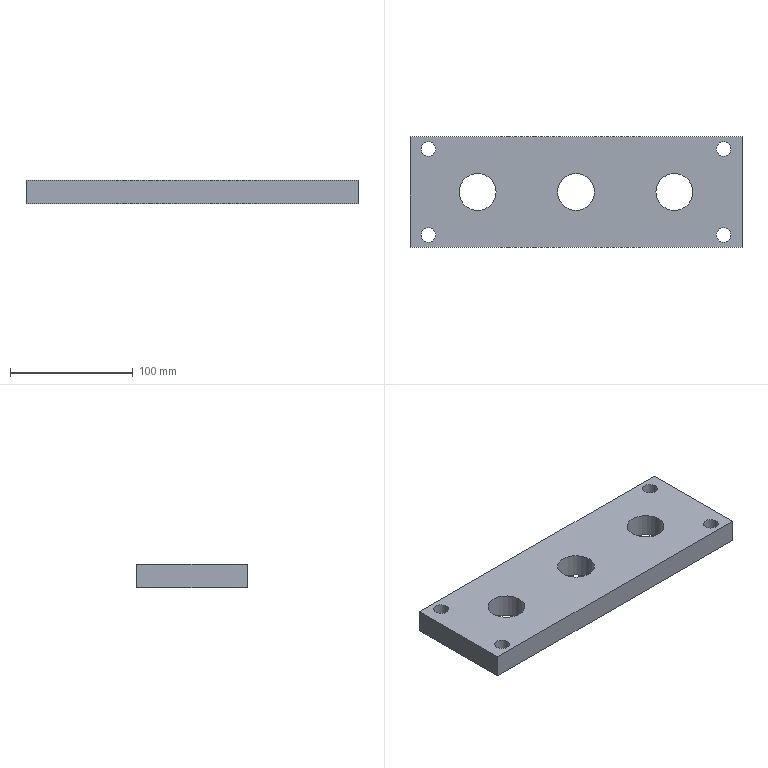Part | NX | features solid 2 | 1 solid | 13 faces | box 270 x 90 x 19 mm | volume 412814 mm3 | cylinder 7 | plane 6 | commonest cylinder face diameters 12 x4 30 x3
STEP:
#1=CARTESIAN_POINT('',(114.,-405.,-144.));
#2=VERTEX_POINT('',#1);
#3=CARTESIAN_POINT('',(120.,-405.,-144.));
#4=DIRECTION('',(0.,0.,1.));
#5=DIRECTION('',(-1.,0.,0.));
#6=AXIS2_PLACEMENT_3D('',#3,#4,#5);
#7=CIRCLE('',#6,6.);
#8=EDGE_CURVE('',#2,#2,#7,.T.);
#9=ORIENTED_EDGE('',*,*,#8,.T.);
#10=EDGE_LOOP('',(#9));
#11=FACE_BOUND('',#10,.T.);
#12=CARTESIAN_POINT('',(114.,-475.,-144.));
#13=VERTEX_POINT('',#12);
#14=CARTESIAN_POINT('',(120.,-475.,-144.));
#15=DIRECTION('',(0.,0.,-1.));
#16=DIRECTION('',(-1.,0.,0.));
#17=AXIS2_PLACEMENT_3D('',#14,#15,#16);
#18=CIRCLE('',#17,6.);
#19=EDGE_CURVE('',#13,#13,#18,.T.);
#20=ORIENTED_EDGE('',*,*,#19,.F.);
#21=EDGE_LOOP('',(#20));
#22=FACE_BOUND('',#21,.T.);
#23=CARTESIAN_POINT('',(-114.,-405.,-144.));
#24=VERTEX_POINT('',#23);
#25=CARTESIAN_POINT('',(-120.,-405.,-144.));
#26=DIRECTION('',(0.,0.,-1.));
#27=DIRECTION('',(1.,0.,0.));
#28=AXIS2_PLACEMENT_3D('',#25,#26,#27);
#29=CIRCLE('',#28,6.);
#30=EDGE_CURVE('',#24,#24,#29,.T.);
#31=ORIENTED_EDGE('',*,*,#30,.F.);
#32=EDGE_LOOP('',(#31));
#33=FACE_BOUND('',#32,.T.);
#34=CARTESIAN_POINT('',(95.,-440.,-144.));
#35=VERTEX_POINT('',#34);
#36=CARTESIAN_POINT('',(80.,-440.,-144.));
#37=DIRECTION('',(0.,0.,-1.));
#38=DIRECTION('',(1.,0.,0.));
#39=AXIS2_PLACEMENT_3D('',#36,#37,#38);
#40=CIRCLE('',#39,15.);
#41=EDGE_CURVE('',#35,#35,#40,.T.);
#42=ORIENTED_EDGE('',*,*,#41,.F.);
#43=EDGE_LOOP('',(#42));
#44=FACE_BOUND('',#43,.T.);
#45=CARTESIAN_POINT('',(-15.,-440.,-144.));
#46=VERTEX_POINT('',#45);
#47=CARTESIAN_POINT('',(0.,-440.,-144.));
#48=DIRECTION('',(0.,0.,1.));
#49=DIRECTION('',(-1.,0.,0.));
#50=AXIS2_PLACEMENT_3D('',#47,#48,#49);
#51=CIRCLE('',#50,15.);
#52=EDGE_CURVE('',#46,#46,#51,.T.);
#53=ORIENTED_EDGE('',*,*,#52,.T.);
#54=EDGE_LOOP('',(#53));
#55=FACE_BOUND('',#54,.T.);
#56=CARTESIAN_POINT('',(-135.,-485.,-144.));
#57=VERTEX_POINT('',#56);
#58=CARTESIAN_POINT('',(-135.,-395.,-144.));
#59=VERTEX_POINT('',#58);
#60=CARTESIAN_POINT('',(-135.,-485.,-144.));
#61=DIRECTION('',(0.,1.,0.));
#62=VECTOR('',#61,1000.);
#63=LINE('',#60,#62);
#64=EDGE_CURVE('',#57,#59,#63,.T.);
#65=ORIENTED_EDGE('',*,*,#64,.T.);
#66=CARTESIAN_POINT('',(135.,-395.,-144.));
#67=VERTEX_POINT('',#66);
#68=CARTESIAN_POINT('',(-135.,-395.,-144.));
#69=DIRECTION('',(1.,0.,0.));
#70=VECTOR('',#69,1000.);
#71=LINE('',#68,#70);
#72=EDGE_CURVE('',#59,#67,#71,.T.);
#73=ORIENTED_EDGE('',*,*,#72,.T.);
#74=CARTESIAN_POINT('',(135.,-485.,-144.));
#75=VERTEX_POINT('',#74);
#76=CARTESIAN_POINT('',(135.,-395.,-144.));
#77=DIRECTION('',(0.,-1.,0.));
#78=VECTOR('',#77,1000.);
#79=LINE('',#76,#78);
#80=EDGE_CURVE('',#67,#75,#79,.T.);
#81=ORIENTED_EDGE('',*,*,#80,.T.);
#82=CARTESIAN_POINT('',(135.,-485.,-144.));
#83=DIRECTION('',(-1.,0.,0.));
#84=VECTOR('',#83,1000.);
#85=LINE('',#82,#84);
#86=EDGE_CURVE('',#75,#57,#85,.T.);
#87=ORIENTED_EDGE('',*,*,#86,.T.);
#88=EDGE_LOOP('',(#65,#73,#81,#87));
#89=FACE_BOUND('',#88,.T.);
#90=CARTESIAN_POINT('',(-95.,-440.,-144.));
#91=VERTEX_POINT('',#90);
#92=CARTESIAN_POINT('',(-80.,-440.,-144.));
#93=DIRECTION('',(0.,0.,1.));
#94=DIRECTION('',(-1.,0.,0.));
#95=AXIS2_PLACEMENT_3D('',#92,#93,#94);
#96=CIRCLE('',#95,15.);
#97=EDGE_CURVE('',#91,#91,#96,.T.);
#98=ORIENTED_EDGE('',*,*,#97,.T.);
#99=EDGE_LOOP('',(#98));
#100=FACE_BOUND('',#99,.T.);
#101=CARTESIAN_POINT('',(-114.,-475.,-144.));
#102=VERTEX_POINT('',#101);
#103=CARTESIAN_POINT('',(-120.,-475.,-144.));
#104=DIRECTION('',(0.,0.,1.));
#105=DIRECTION('',(1.,0.,0.));
#106=AXIS2_PLACEMENT_3D('',#103,#104,#105);
#107=CIRCLE('',#106,6.);
#108=EDGE_CURVE('',#102,#102,#107,.T.);
#109=ORIENTED_EDGE('',*,*,#108,.T.);
#110=EDGE_LOOP('',(#109));
#111=FACE_BOUND('',#110,.T.);
#112=CARTESIAN_POINT('',(-135.,-395.,-144.));
#113=DIRECTION('',(0.,0.,1.));
#114=DIRECTION('',(-1.,0.,0.));
#115=AXIS2_PLACEMENT_3D('',#112,#113,#114);
#116=PLANE('',#115);
#117=ADVANCED_FACE('',(#11,#22,#33,#44,#55,#89,#100,#111),#116,.F.);
#118=CARTESIAN_POINT('',(114.,-405.,-125.));
#119=VERTEX_POINT('',#118);
#120=CARTESIAN_POINT('',(120.,-405.,-125.));
#121=DIRECTION('',(0.,0.,1.));
#122=DIRECTION('',(-1.,0.,0.));
#123=AXIS2_PLACEMENT_3D('',#120,#121,#122);
#124=CIRCLE('',#123,6.);
#125=EDGE_CURVE('',#119,#119,#124,.T.);
#126=ORIENTED_EDGE('',*,*,#125,.F.);
#127=EDGE_LOOP('',(#126));
#128=FACE_BOUND('',#127,.T.);
#129=CARTESIAN_POINT('',(114.,-475.,-125.));
#130=VERTEX_POINT('',#129);
#131=CARTESIAN_POINT('',(120.,-475.,-125.));
#132=DIRECTION('',(0.,0.,-1.));
#133=DIRECTION('',(-1.,0.,0.));
#134=AXIS2_PLACEMENT_3D('',#131,#132,#133);
#135=CIRCLE('',#134,6.);
#136=EDGE_CURVE('',#130,#130,#135,.T.);
#137=ORIENTED_EDGE('',*,*,#136,.T.);
#138=EDGE_LOOP('',(#137));
#139=FACE_BOUND('',#138,.T.);
#140=CARTESIAN_POINT('',(-114.,-405.,-125.));
#141=VERTEX_POINT('',#140);
#142=CARTESIAN_POINT('',(-120.,-405.,-125.));
#143=DIRECTION('',(0.,0.,-1.));
#144=DIRECTION('',(1.,0.,0.));
#145=AXIS2_PLACEMENT_3D('',#142,#143,#144);
#146=CIRCLE('',#145,6.);
#147=EDGE_CURVE('',#141,#141,#146,.T.);
#148=ORIENTED_EDGE('',*,*,#147,.T.);
#149=EDGE_LOOP('',(#148));
#150=FACE_BOUND('',#149,.T.);
#151=CARTESIAN_POINT('',(95.,-440.,-125.));
#152=VERTEX_POINT('',#151);
#153=CARTESIAN_POINT('',(80.,-440.,-125.));
#154=DIRECTION('',(0.,0.,-1.));
#155=DIRECTION('',(1.,0.,0.));
#156=AXIS2_PLACEMENT_3D('',#153,#154,#155);
#157=CIRCLE('',#156,15.);
#158=EDGE_CURVE('',#152,#152,#157,.T.);
#159=ORIENTED_EDGE('',*,*,#158,.T.);
#160=EDGE_LOOP('',(#159));
#161=FACE_BOUND('',#160,.T.);
#162=CARTESIAN_POINT('',(-15.,-440.,-125.));
#163=VERTEX_POINT('',#162);
#164=CARTESIAN_POINT('',(0.,-440.,-125.));
#165=DIRECTION('',(0.,0.,1.));
#166=DIRECTION('',(-1.,0.,0.));
#167=AXIS2_PLACEMENT_3D('',#164,#165,#166);
#168=CIRCLE('',#167,15.);
#169=EDGE_CURVE('',#163,#163,#168,.T.);
#170=ORIENTED_EDGE('',*,*,#169,.F.);
#171=EDGE_LOOP('',(#170));
#172=FACE_BOUND('',#171,.T.);
#173=CARTESIAN_POINT('',(-135.,-485.,-125.));
#174=VERTEX_POINT('',#173);
#175=CARTESIAN_POINT('',(-135.,-395.,-125.));
#176=VERTEX_POINT('',#175);
#177=CARTESIAN_POINT('',(-135.,-485.,-125.));
#178=DIRECTION('',(0.,1.,0.));
#179=VECTOR('',#178,1000.);
#180=LINE('',#177,#179);
#181=EDGE_CURVE('',#174,#176,#180,.T.);
#182=ORIENTED_EDGE('',*,*,#181,.F.);
#183=CARTESIAN_POINT('',(135.,-485.,-125.));
#184=VERTEX_POINT('',#183);
#185=CARTESIAN_POINT('',(135.,-485.,-125.));
#186=DIRECTION('',(-1.,0.,0.));
#187=VECTOR('',#186,1000.);
#188=LINE('',#185,#187);
#189=EDGE_CURVE('',#184,#174,#188,.T.);
#190=ORIENTED_EDGE('',*,*,#189,.F.);
#191=CARTESIAN_POINT('',(135.,-395.,-125.));
#192=VERTEX_POINT('',#191);
#193=CARTESIAN_POINT('',(135.,-395.,-125.));
#194=DIRECTION('',(0.,-1.,0.));
#195=VECTOR('',#194,1000.);
#196=LINE('',#193,#195);
#197=EDGE_CURVE('',#192,#184,#196,.T.);
#198=ORIENTED_EDGE('',*,*,#197,.F.);
#199=CARTESIAN_POINT('',(-135.,-395.,-125.));
#200=DIRECTION('',(1.,0.,0.));
#201=VECTOR('',#200,1000.);
#202=LINE('',#199,#201);
#203=EDGE_CURVE('',#176,#192,#202,.T.);
#204=ORIENTED_EDGE('',*,*,#203,.F.);
#205=EDGE_LOOP('',(#182,#190,#198,#204));
#206=FACE_BOUND('',#205,.T.);
#207=CARTESIAN_POINT('',(-95.,-440.,-125.));
#208=VERTEX_POINT('',#207);
#209=CARTESIAN_POINT('',(-80.,-440.,-125.));
#210=DIRECTION('',(0.,0.,1.));
#211=DIRECTION('',(-1.,0.,0.));
#212=AXIS2_PLACEMENT_3D('',#209,#210,#211);
#213=CIRCLE('',#212,15.);
#214=EDGE_CURVE('',#208,#208,#213,.T.);
#215=ORIENTED_EDGE('',*,*,#214,.F.);
#216=EDGE_LOOP('',(#215));
#217=FACE_BOUND('',#216,.T.);
#218=CARTESIAN_POINT('',(-114.,-475.,-125.));
#219=VERTEX_POINT('',#218);
#220=CARTESIAN_POINT('',(-120.,-475.,-125.));
#221=DIRECTION('',(0.,0.,1.));
#222=DIRECTION('',(1.,0.,0.));
#223=AXIS2_PLACEMENT_3D('',#220,#221,#222);
#224=CIRCLE('',#223,6.);
#225=EDGE_CURVE('',#219,#219,#224,.T.);
#226=ORIENTED_EDGE('',*,*,#225,.F.);
#227=EDGE_LOOP('',(#226));
#228=FACE_BOUND('',#227,.T.);
#229=CARTESIAN_POINT('',(-135.,-395.,-125.));
#230=DIRECTION('',(0.,0.,1.));
#231=DIRECTION('',(-1.,0.,0.));
#232=AXIS2_PLACEMENT_3D('',#229,#230,#231);
#233=PLANE('',#232);
#234=ADVANCED_FACE('',(#128,#139,#150,#161,#172,#206,#217,#228),#233,.T.);
#235=ORIENTED_EDGE('',*,*,#181,.T.);
#236=CARTESIAN_POINT('',(-135.,-395.,-144.));
#237=DIRECTION('',(0.,0.,1.));
#238=VECTOR('',#237,1000.);
#239=LINE('',#236,#238);
#240=EDGE_CURVE('',#59,#176,#239,.T.);
#241=ORIENTED_EDGE('',*,*,#240,.F.);
#242=ORIENTED_EDGE('',*,*,#64,.F.);
#243=CARTESIAN_POINT('',(-135.,-485.,-144.));
#244=DIRECTION('',(0.,0.,1.));
#245=VECTOR('',#244,1000.);
#246=LINE('',#243,#245);
#247=EDGE_CURVE('',#57,#174,#246,.T.);
#248=ORIENTED_EDGE('',*,*,#247,.T.);
#249=EDGE_LOOP('',(#235,#241,#242,#248));
#250=FACE_BOUND('',#249,.T.);
#251=CARTESIAN_POINT('',(-135.,-485.,-144.));
#252=DIRECTION('',(-1.,0.,0.));
#253=DIRECTION('',(0.,0.,-1.));
#254=AXIS2_PLACEMENT_3D('',#251,#252,#253);
#255=PLANE('',#254);
#256=ADVANCED_FACE('',(#250),#255,.T.);
#257=ORIENTED_EDGE('',*,*,#203,.T.);
#258=CARTESIAN_POINT('',(135.,-395.,-144.));
#259=DIRECTION('',(0.,0.,1.));
#260=VECTOR('',#259,1000.);
#261=LINE('',#258,#260);
#262=EDGE_CURVE('',#67,#192,#261,.T.);
#263=ORIENTED_EDGE('',*,*,#262,.F.);
#264=ORIENTED_EDGE('',*,*,#72,.F.);
#265=ORIENTED_EDGE('',*,*,#240,.T.);
#266=EDGE_LOOP('',(#257,#263,#264,#265));
#267=FACE_BOUND('',#266,.T.);
#268=CARTESIAN_POINT('',(-135.,-395.,-144.));
#269=DIRECTION('',(0.,1.,0.));
#270=DIRECTION('',(0.,0.,-1.));
#271=AXIS2_PLACEMENT_3D('',#268,#269,#270);
#272=PLANE('',#271);
#273=ADVANCED_FACE('',(#267),#272,.T.);
#274=ORIENTED_EDGE('',*,*,#197,.T.);
#275=CARTESIAN_POINT('',(135.,-485.,-144.));
#276=DIRECTION('',(0.,0.,1.));
#277=VECTOR('',#276,1000.);
#278=LINE('',#275,#277);
#279=EDGE_CURVE('',#75,#184,#278,.T.);
#280=ORIENTED_EDGE('',*,*,#279,.F.);
#281=ORIENTED_EDGE('',*,*,#80,.F.);
#282=ORIENTED_EDGE('',*,*,#262,.T.);
#283=EDGE_LOOP('',(#274,#280,#281,#282));
#284=FACE_BOUND('',#283,.T.);
#285=CARTESIAN_POINT('',(135.,-395.,-144.));
#286=DIRECTION('',(1.,0.,0.));
#287=DIRECTION('',(0.,0.,1.));
#288=AXIS2_PLACEMENT_3D('',#285,#286,#287);
#289=PLANE('',#288);
#290=ADVANCED_FACE('',(#284),#289,.T.);
#291=ORIENTED_EDGE('',*,*,#189,.T.);
#292=ORIENTED_EDGE('',*,*,#247,.F.);
#293=ORIENTED_EDGE('',*,*,#86,.F.);
#294=ORIENTED_EDGE('',*,*,#279,.T.);
#295=EDGE_LOOP('',(#291,#292,#293,#294));
#296=FACE_BOUND('',#295,.T.);
#297=CARTESIAN_POINT('',(135.,-485.,-144.));
#298=DIRECTION('',(0.,-1.,0.));
#299=DIRECTION('',(0.,0.,1.));
#300=AXIS2_PLACEMENT_3D('',#297,#298,#299);
#301=PLANE('',#300);
#302=ADVANCED_FACE('',(#296),#301,.T.);
#303=ORIENTED_EDGE('',*,*,#52,.F.);
#304=EDGE_LOOP('',(#303));
#305=FACE_BOUND('',#304,.T.);
#306=ORIENTED_EDGE('',*,*,#169,.T.);
#307=EDGE_LOOP('',(#306));
#308=FACE_BOUND('',#307,.T.);
#309=CARTESIAN_POINT('',(0.,-440.,-144.));
#310=DIRECTION('',(0.,0.,1.));
#311=DIRECTION('',(-1.,0.,0.));
#312=AXIS2_PLACEMENT_3D('',#309,#310,#311);
#313=CYLINDRICAL_SURFACE('',#312,15.);
#314=ADVANCED_FACE('',(#305,#308),#313,.F.);
#315=ORIENTED_EDGE('',*,*,#41,.T.);
#316=EDGE_LOOP('',(#315));
#317=FACE_BOUND('',#316,.T.);
#318=ORIENTED_EDGE('',*,*,#158,.F.);
#319=EDGE_LOOP('',(#318));
#320=FACE_BOUND('',#319,.T.);
#321=CARTESIAN_POINT('',(80.,-440.,-144.));
#322=DIRECTION('',(0.,0.,1.));
#323=DIRECTION('',(-1.,0.,0.));
#324=AXIS2_PLACEMENT_3D('',#321,#322,#323);
#325=CYLINDRICAL_SURFACE('',#324,15.);
#326=ADVANCED_FACE('',(#317,#320),#325,.F.);
#327=ORIENTED_EDGE('',*,*,#97,.F.);
#328=EDGE_LOOP('',(#327));
#329=FACE_BOUND('',#328,.T.);
#330=ORIENTED_EDGE('',*,*,#214,.T.);
#331=EDGE_LOOP('',(#330));
#332=FACE_BOUND('',#331,.T.);
#333=CARTESIAN_POINT('',(-80.,-440.,-144.));
#334=DIRECTION('',(0.,0.,1.));
#335=DIRECTION('',(-1.,0.,0.));
#336=AXIS2_PLACEMENT_3D('',#333,#334,#335);
#337=CYLINDRICAL_SURFACE('',#336,15.);
#338=ADVANCED_FACE('',(#329,#332),#337,.F.);
#339=ORIENTED_EDGE('',*,*,#30,.T.);
#340=EDGE_LOOP('',(#339));
#341=FACE_BOUND('',#340,.T.);
#342=ORIENTED_EDGE('',*,*,#147,.F.);
#343=EDGE_LOOP('',(#342));
#344=FACE_BOUND('',#343,.T.);
#345=CARTESIAN_POINT('',(-120.,-405.,-144.));
#346=DIRECTION('',(0.,0.,1.));
#347=DIRECTION('',(-1.,0.,0.));
#348=AXIS2_PLACEMENT_3D('',#345,#346,#347);
#349=CYLINDRICAL_SURFACE('',#348,6.);
#350=ADVANCED_FACE('',(#341,#344),#349,.F.);
#351=ORIENTED_EDGE('',*,*,#19,.T.);
#352=EDGE_LOOP('',(#351));
#353=FACE_BOUND('',#352,.T.);
#354=ORIENTED_EDGE('',*,*,#136,.F.);
#355=EDGE_LOOP('',(#354));
#356=FACE_BOUND('',#355,.T.);
#357=CARTESIAN_POINT('',(120.,-475.,-144.));
#358=DIRECTION('',(0.,0.,1.));
#359=DIRECTION('',(-1.,0.,0.));
#360=AXIS2_PLACEMENT_3D('',#357,#358,#359);
#361=CYLINDRICAL_SURFACE('',#360,6.);
#362=ADVANCED_FACE('',(#353,#356),#361,.F.);
#363=ORIENTED_EDGE('',*,*,#8,.F.);
#364=EDGE_LOOP('',(#363));
#365=FACE_BOUND('',#364,.T.);
#366=ORIENTED_EDGE('',*,*,#125,.T.);
#367=EDGE_LOOP('',(#366));
#368=FACE_BOUND('',#367,.T.);
#369=CARTESIAN_POINT('',(120.,-405.,-144.));
#370=DIRECTION('',(0.,0.,1.));
#371=DIRECTION('',(-1.,0.,0.));
#372=AXIS2_PLACEMENT_3D('',#369,#370,#371);
#373=CYLINDRICAL_SURFACE('',#372,6.);
#374=ADVANCED_FACE('',(#365,#368),#373,.F.);
#375=ORIENTED_EDGE('',*,*,#108,.F.);
#376=EDGE_LOOP('',(#375));
#377=FACE_BOUND('',#376,.T.);
#378=ORIENTED_EDGE('',*,*,#225,.T.);
#379=EDGE_LOOP('',(#378));
#380=FACE_BOUND('',#379,.T.);
#381=CARTESIAN_POINT('',(-120.,-475.,-144.));
#382=DIRECTION('',(0.,0.,1.));
#383=DIRECTION('',(-1.,0.,0.));
#384=AXIS2_PLACEMENT_3D('',#381,#382,#383);
#385=CYLINDRICAL_SURFACE('',#384,6.);
#386=ADVANCED_FACE('',(#377,#380),#385,.F.);
#387=CLOSED_SHELL('',(#117,#234,#256,#273,#290,#302,#314,#326,#338,#350,#362,#374,#386));
#388=MANIFOLD_SOLID_BREP('',#387);
#389=(LENGTH_UNIT()NAMED_UNIT(*)SI_UNIT(.MILLI.,.METRE.));
#390=UNCERTAINTY_MEASURE_WITH_UNIT(LENGTH_MEASURE(0.00001),#389,'','');
#391=(NAMED_UNIT(*)PLANE_ANGLE_UNIT()SI_UNIT($,.RADIAN.));
#392=(NAMED_UNIT(*)SI_UNIT($,.STERADIAN.)SOLID_ANGLE_UNIT());
#393=(GEOMETRIC_REPRESENTATION_CONTEXT(3)GLOBAL_UNCERTAINTY_ASSIGNED_CONTEXT((#390))GLOBAL_UNIT_ASSIGNED_CONTEXT((#389,#391,#392))REPRESENTATION_CONTEXT('',''));
#394=ADVANCED_BREP_SHAPE_REPRESENTATION('',(#388),#393);